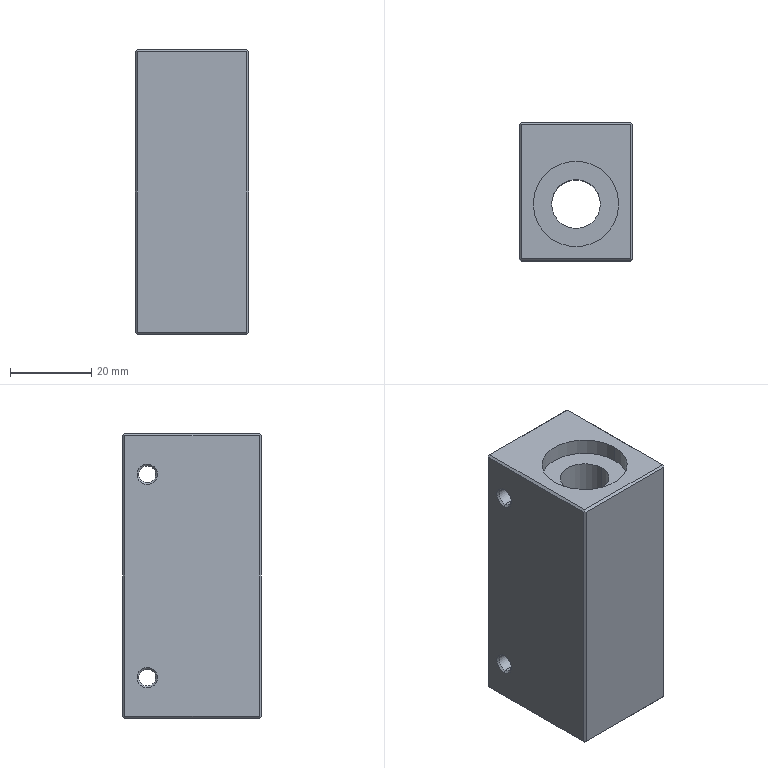Part | SolidWorks | features RevCut 7, ICE 2, Extrusion 1 | 1 solid | 50 faces | box 28 x 34 x 70 mm | volume 55264 mm3 | plane 24 | cylinder 18 | cone 8 | commonest cylinder face diameters 4.134 x4 4.917 x4 8 x4 21 x4 12 x2
STEP:
#1=CARTESIAN_POINT('',(8.,14.,22.933));
#2=VERTEX_POINT('',#1);
#3=CARTESIAN_POINT('',(8.,14.,27.067));
#4=VERTEX_POINT('',#3);
#5=CARTESIAN_POINT('',(8.,14.,25.));
#6=DIRECTION('',(-1.,0.,0.));
#7=DIRECTION('',(0.,0.,1.));
#8=AXIS2_PLACEMENT_3D('',#5,#6,#7);
#9=CIRCLE('',#8,2.067);
#10=EDGE_CURVE('',#2,#4,#9,.T.);
#11=ORIENTED_EDGE('',*,*,#10,.F.);
#12=CARTESIAN_POINT('',(-13.567,14.,22.933));
#13=VERTEX_POINT('',#12);
#14=CARTESIAN_POINT('',(8.,14.,22.933));
#15=DIRECTION('',(-1.,0.,0.));
#16=VECTOR('',#15,1000.);
#17=LINE('',#14,#16);
#18=EDGE_CURVE('',#2,#13,#17,.T.);
#19=ORIENTED_EDGE('',*,*,#18,.T.);
#20=CARTESIAN_POINT('',(-13.567,14.,27.067));
#21=VERTEX_POINT('',#20);
#22=CARTESIAN_POINT('',(-13.567,14.,25.));
#23=DIRECTION('',(-1.,0.,0.));
#24=DIRECTION('',(0.,0.,1.));
#25=AXIS2_PLACEMENT_3D('',#22,#23,#24);
#26=CIRCLE('',#25,2.067);
#27=EDGE_CURVE('',#13,#21,#26,.T.);
#28=ORIENTED_EDGE('',*,*,#27,.T.);
#29=CARTESIAN_POINT('',(8.,14.,27.067));
#30=DIRECTION('',(-1.,0.,0.));
#31=VECTOR('',#30,1000.);
#32=LINE('',#29,#31);
#33=EDGE_CURVE('',#4,#21,#32,.T.);
#34=ORIENTED_EDGE('',*,*,#33,.F.);
#35=EDGE_LOOP('',(#11,#19,#28,#34));
#36=FACE_OUTER_BOUND('',#35,.T.);
#37=CARTESIAN_POINT('',(8.,14.,25.));
#38=DIRECTION('',(-1.,0.,0.));
#39=DIRECTION('',(0.,0.,1.));
#40=AXIS2_PLACEMENT_3D('',#37,#38,#39);
#41=CYLINDRICAL_SURFACE('',#40,2.067);
#42=ADVANCED_FACE('',(#36),#41,.F.);
#43=ORIENTED_EDGE('',*,*,#27,.F.);
#44=CARTESIAN_POINT('',(-14.,14.,22.5));
#45=VERTEX_POINT('',#44);
#46=CARTESIAN_POINT('',(-13.567,14.,22.933));
#47=DIRECTION('',(-0.7071,0.,-0.7071));
#48=VECTOR('',#47,1000.);
#49=LINE('',#46,#48);
#50=EDGE_CURVE('',#13,#45,#49,.T.);
#51=ORIENTED_EDGE('',*,*,#50,.T.);
#52=CARTESIAN_POINT('',(-14.,14.,27.5));
#53=VERTEX_POINT('',#52);
#54=CARTESIAN_POINT('',(-14.,14.,25.));
#55=DIRECTION('',(-1.,0.,0.));
#56=DIRECTION('',(0.,0.,1.));
#57=AXIS2_PLACEMENT_3D('',#54,#55,#56);
#58=CIRCLE('',#57,2.5);
#59=EDGE_CURVE('',#45,#53,#58,.T.);
#60=ORIENTED_EDGE('',*,*,#59,.T.);
#61=CARTESIAN_POINT('',(-13.567,14.,27.067));
#62=DIRECTION('',(-0.7071,0.,0.7071));
#63=VECTOR('',#62,1000.);
#64=LINE('',#61,#63);
#65=EDGE_CURVE('',#21,#53,#64,.T.);
#66=ORIENTED_EDGE('',*,*,#65,.F.);
#67=EDGE_LOOP('',(#43,#51,#60,#66));
#68=FACE_OUTER_BOUND('',#67,.T.);
#69=CARTESIAN_POINT('',(-13.567,14.,25.));
#70=DIRECTION('',(-1.,0.,0.));
#71=DIRECTION('',(0.,0.,1.));
#72=AXIS2_PLACEMENT_3D('',#69,#70,#71);
#73=CONICAL_SURFACE('',#72,2.067,0.7854);
#74=ADVANCED_FACE('',(#68),#73,.F.);
#75=CARTESIAN_POINT('',(8.,14.,-27.067));
#76=VERTEX_POINT('',#75);
#77=CARTESIAN_POINT('',(8.,14.,-22.933));
#78=VERTEX_POINT('',#77);
#79=CARTESIAN_POINT('',(8.,14.,-25.));
#80=DIRECTION('',(-1.,0.,0.));
#81=DIRECTION('',(0.,0.,1.));
#82=AXIS2_PLACEMENT_3D('',#79,#80,#81);
#83=CIRCLE('',#82,2.067);
#84=EDGE_CURVE('',#76,#78,#83,.T.);
#85=ORIENTED_EDGE('',*,*,#84,.F.);
#86=CARTESIAN_POINT('',(-13.567,14.,-27.067));
#87=VERTEX_POINT('',#86);
#88=CARTESIAN_POINT('',(8.,14.,-27.067));
#89=DIRECTION('',(-1.,0.,0.));
#90=VECTOR('',#89,1000.);
#91=LINE('',#88,#90);
#92=EDGE_CURVE('',#76,#87,#91,.T.);
#93=ORIENTED_EDGE('',*,*,#92,.T.);
#94=CARTESIAN_POINT('',(-13.567,14.,-22.933));
#95=VERTEX_POINT('',#94);
#96=CARTESIAN_POINT('',(-13.567,14.,-25.));
#97=DIRECTION('',(-1.,0.,0.));
#98=DIRECTION('',(0.,0.,1.));
#99=AXIS2_PLACEMENT_3D('',#96,#97,#98);
#100=CIRCLE('',#99,2.067);
#101=EDGE_CURVE('',#87,#95,#100,.T.);
#102=ORIENTED_EDGE('',*,*,#101,.T.);
#103=CARTESIAN_POINT('',(8.,14.,-22.933));
#104=DIRECTION('',(-1.,0.,0.));
#105=VECTOR('',#104,1000.);
#106=LINE('',#103,#105);
#107=EDGE_CURVE('',#78,#95,#106,.T.);
#108=ORIENTED_EDGE('',*,*,#107,.F.);
#109=EDGE_LOOP('',(#85,#93,#102,#108));
#110=FACE_OUTER_BOUND('',#109,.T.);
#111=CARTESIAN_POINT('',(8.,14.,-25.));
#112=DIRECTION('',(-1.,0.,0.));
#113=DIRECTION('',(0.,0.,1.));
#114=AXIS2_PLACEMENT_3D('',#111,#112,#113);
#115=CYLINDRICAL_SURFACE('',#114,2.067);
#116=ADVANCED_FACE('',(#110),#115,.F.);
#117=ORIENTED_EDGE('',*,*,#101,.F.);
#118=CARTESIAN_POINT('',(-14.,14.,-27.5));
#119=VERTEX_POINT('',#118);
#120=CARTESIAN_POINT('',(-13.567,14.,-27.067));
#121=DIRECTION('',(-0.7071,0.,-0.7071));
#122=VECTOR('',#121,1000.);
#123=LINE('',#120,#122);
#124=EDGE_CURVE('',#87,#119,#123,.T.);
#125=ORIENTED_EDGE('',*,*,#124,.T.);
#126=CARTESIAN_POINT('',(-14.,14.,-22.5));
#127=VERTEX_POINT('',#126);
#128=CARTESIAN_POINT('',(-14.,14.,-25.));
#129=DIRECTION('',(-1.,0.,0.));
#130=DIRECTION('',(0.,0.,1.));
#131=AXIS2_PLACEMENT_3D('',#128,#129,#130);
#132=CIRCLE('',#131,2.5);
#133=EDGE_CURVE('',#119,#127,#132,.T.);
#134=ORIENTED_EDGE('',*,*,#133,.T.);
#135=CARTESIAN_POINT('',(-13.567,14.,-22.933));
#136=DIRECTION('',(-0.7071,0.,0.7071));
#137=VECTOR('',#136,1000.);
#138=LINE('',#135,#137);
#139=EDGE_CURVE('',#95,#127,#138,.T.);
#140=ORIENTED_EDGE('',*,*,#139,.F.);
#141=EDGE_LOOP('',(#117,#125,#134,#140));
#142=FACE_OUTER_BOUND('',#141,.T.);
#143=CARTESIAN_POINT('',(-13.567,14.,-25.));
#144=DIRECTION('',(-1.,0.,0.));
#145=DIRECTION('',(0.,0.,1.));
#146=AXIS2_PLACEMENT_3D('',#143,#144,#145);
#147=CONICAL_SURFACE('',#146,2.067,0.7854);
#148=ADVANCED_FACE('',(#142),#147,.F.);
#149=CARTESIAN_POINT('',(0.,10.92,15.541));
#150=VERTEX_POINT('',#149);
#151=CARTESIAN_POINT('',(0.,10.92,20.459));
#152=VERTEX_POINT('',#151);
#153=CARTESIAN_POINT('',(0.,10.92,18.));
#154=DIRECTION('',(0.,1.,0.));
#155=DIRECTION('',(0.,0.,1.));
#156=AXIS2_PLACEMENT_3D('',#153,#154,#155);
#157=CIRCLE('',#156,2.459);
#158=EDGE_CURVE('',#150,#152,#157,.T.);
#159=ORIENTED_EDGE('',*,*,#158,.F.);
#160=CARTESIAN_POINT('',(0.,19.459,15.541));
#161=VERTEX_POINT('',#160);
#162=CARTESIAN_POINT('',(0.,10.92,15.541));
#163=DIRECTION('',(0.,1.,0.));
#164=VECTOR('',#163,1000.);
#165=LINE('',#162,#164);
#166=EDGE_CURVE('',#150,#161,#165,.T.);
#167=ORIENTED_EDGE('',*,*,#166,.T.);
#168=CARTESIAN_POINT('',(0.,19.459,20.459));
#169=VERTEX_POINT('',#168);
#170=CARTESIAN_POINT('',(0.,19.459,18.));
#171=DIRECTION('',(0.,1.,0.));
#172=DIRECTION('',(0.,0.,1.));
#173=AXIS2_PLACEMENT_3D('',#170,#171,#172);
#174=CIRCLE('',#173,2.459);
#175=EDGE_CURVE('',#161,#169,#174,.T.);
#176=ORIENTED_EDGE('',*,*,#175,.T.);
#177=CARTESIAN_POINT('',(0.,10.92,20.459));
#178=DIRECTION('',(0.,1.,0.));
#179=VECTOR('',#178,1000.);
#180=LINE('',#177,#179);
#181=EDGE_CURVE('',#152,#169,#180,.T.);
#182=ORIENTED_EDGE('',*,*,#181,.F.);
#183=EDGE_LOOP('',(#159,#167,#176,#182));
#184=FACE_OUTER_BOUND('',#183,.T.);
#185=CARTESIAN_POINT('',(0.,10.92,18.));
#186=DIRECTION('',(0.,1.,0.));
#187=DIRECTION('',(0.,0.,1.));
#188=AXIS2_PLACEMENT_3D('',#185,#186,#187);
#189=CYLINDRICAL_SURFACE('',#188,2.459);
#190=ADVANCED_FACE('',(#184),#189,.F.);
#191=ORIENTED_EDGE('',*,*,#175,.F.);
#192=CARTESIAN_POINT('',(0.,20.,15.));
#193=VERTEX_POINT('',#192);
#194=CARTESIAN_POINT('',(0.,19.459,15.541));
#195=DIRECTION('',(0.,0.7071,-0.7071));
#196=VECTOR('',#195,1000.);
#197=LINE('',#194,#196);
#198=EDGE_CURVE('',#161,#193,#197,.T.);
#199=ORIENTED_EDGE('',*,*,#198,.T.);
#200=CARTESIAN_POINT('',(0.,20.,21.));
#201=VERTEX_POINT('',#200);
#202=CARTESIAN_POINT('',(0.,20.,18.));
#203=DIRECTION('',(0.,1.,0.));
#204=DIRECTION('',(0.,0.,1.));
#205=AXIS2_PLACEMENT_3D('',#202,#203,#204);
#206=CIRCLE('',#205,3.);
#207=EDGE_CURVE('',#193,#201,#206,.T.);
#208=ORIENTED_EDGE('',*,*,#207,.T.);
#209=CARTESIAN_POINT('',(0.,19.459,20.459));
#210=DIRECTION('',(0.,0.7071,0.7071));
#211=VECTOR('',#210,1000.);
#212=LINE('',#209,#211);
#213=EDGE_CURVE('',#169,#201,#212,.T.);
#214=ORIENTED_EDGE('',*,*,#213,.F.);
#215=EDGE_LOOP('',(#191,#199,#208,#214));
#216=FACE_OUTER_BOUND('',#215,.T.);
#217=CARTESIAN_POINT('',(0.,19.459,18.));
#218=DIRECTION('',(0.,1.,0.));
#219=DIRECTION('',(0.,0.,1.));
#220=AXIS2_PLACEMENT_3D('',#217,#218,#219);
#221=CONICAL_SURFACE('',#220,2.459,0.7854);
#222=ADVANCED_FACE('',(#216),#221,.F.);
#223=CARTESIAN_POINT('',(0.,10.92,-20.459));
#224=VERTEX_POINT('',#223);
#225=CARTESIAN_POINT('',(0.,10.92,-15.542));
#226=VERTEX_POINT('',#225);
#227=CARTESIAN_POINT('',(0.,10.92,-18.));
#228=DIRECTION('',(0.,1.,0.));
#229=DIRECTION('',(0.,0.,1.));
#230=AXIS2_PLACEMENT_3D('',#227,#228,#229);
#231=CIRCLE('',#230,2.458);
#232=EDGE_CURVE('',#224,#226,#231,.T.);
#233=ORIENTED_EDGE('',*,*,#232,.F.);
#234=CARTESIAN_POINT('',(0.,19.459,-20.459));
#235=VERTEX_POINT('',#234);
#236=CARTESIAN_POINT('',(0.,10.92,-20.459));
#237=DIRECTION('',(0.,1.,0.));
#238=VECTOR('',#237,1000.);
#239=LINE('',#236,#238);
#240=EDGE_CURVE('',#224,#235,#239,.T.);
#241=ORIENTED_EDGE('',*,*,#240,.T.);
#242=CARTESIAN_POINT('',(0.,19.459,-15.542));
#243=VERTEX_POINT('',#242);
#244=CARTESIAN_POINT('',(0.,19.459,-18.));
#245=DIRECTION('',(0.,1.,0.));
#246=DIRECTION('',(0.,0.,1.));
#247=AXIS2_PLACEMENT_3D('',#244,#245,#246);
#248=CIRCLE('',#247,2.458);
#249=EDGE_CURVE('',#235,#243,#248,.T.);
#250=ORIENTED_EDGE('',*,*,#249,.T.);
#251=CARTESIAN_POINT('',(0.,10.92,-15.542));
#252=DIRECTION('',(0.,1.,0.));
#253=VECTOR('',#252,1000.);
#254=LINE('',#251,#253);
#255=EDGE_CURVE('',#226,#243,#254,.T.);
#256=ORIENTED_EDGE('',*,*,#255,.F.);
#257=EDGE_LOOP('',(#233,#241,#250,#256));
#258=FACE_OUTER_BOUND('',#257,.T.);
#259=CARTESIAN_POINT('',(0.,10.92,-18.));
#260=DIRECTION('',(0.,1.,0.));
#261=DIRECTION('',(0.,0.,1.));
#262=AXIS2_PLACEMENT_3D('',#259,#260,#261);
#263=CYLINDRICAL_SURFACE('',#262,2.458);
#264=ADVANCED_FACE('',(#258),#263,.F.);
#265=ORIENTED_EDGE('',*,*,#249,.F.);
#266=CARTESIAN_POINT('',(0.,20.,-21.));
#267=VERTEX_POINT('',#266);
#268=CARTESIAN_POINT('',(0.,19.459,-20.459));
#269=DIRECTION('',(0.,0.7071,-0.7071));
#270=VECTOR('',#269,1000.);
#271=LINE('',#268,#270);
#272=EDGE_CURVE('',#235,#267,#271,.T.);
#273=ORIENTED_EDGE('',*,*,#272,.T.);
#274=CARTESIAN_POINT('',(0.,20.,-15.));
#275=VERTEX_POINT('',#274);
#276=CARTESIAN_POINT('',(0.,20.,-18.));
#277=DIRECTION('',(0.,1.,0.));
#278=DIRECTION('',(0.,0.,1.));
#279=AXIS2_PLACEMENT_3D('',#276,#277,#278);
#280=CIRCLE('',#279,3.);
#281=EDGE_CURVE('',#267,#275,#280,.T.);
#282=ORIENTED_EDGE('',*,*,#281,.T.);
#283=CARTESIAN_POINT('',(0.,19.459,-15.542));
#284=DIRECTION('',(0.,0.7071,0.7071));
#285=VECTOR('',#284,1000.);
#286=LINE('',#283,#285);
#287=EDGE_CURVE('',#243,#275,#286,.T.);
#288=ORIENTED_EDGE('',*,*,#287,.F.);
#289=EDGE_LOOP('',(#265,#273,#282,#288));
#290=FACE_OUTER_BOUND('',#289,.T.);
#291=CARTESIAN_POINT('',(0.,19.459,-18.));
#292=DIRECTION('',(0.,1.,0.));
#293=DIRECTION('',(0.,0.,1.));
#294=AXIS2_PLACEMENT_3D('',#291,#292,#293);
#295=CONICAL_SURFACE('',#294,2.458,0.7854);
#296=ADVANCED_FACE('',(#290),#295,.F.);
#297=CARTESIAN_POINT('',(14.,14.,-29.));
#298=VERTEX_POINT('',#297);
#299=CARTESIAN_POINT('',(14.,14.,-21.));
#300=VERTEX_POINT('',#299);
#301=CARTESIAN_POINT('',(14.,14.,-25.));
#302=DIRECTION('',(-1.,0.,0.));
#303=DIRECTION('',(0.,0.,1.));
#304=AXIS2_PLACEMENT_3D('',#301,#302,#303);
#305=CIRCLE('',#304,4.);
#306=EDGE_CURVE('',#298,#300,#305,.T.);
#307=ORIENTED_EDGE('',*,*,#306,.F.);
#308=CARTESIAN_POINT('',(8.,14.,-29.));
#309=VERTEX_POINT('',#308);
#310=CARTESIAN_POINT('',(14.,14.,-29.));
#311=DIRECTION('',(-1.,0.,0.));
#312=VECTOR('',#311,1000.);
#313=LINE('',#310,#312);
#314=EDGE_CURVE('',#298,#309,#313,.T.);
#315=ORIENTED_EDGE('',*,*,#314,.T.);
#316=CARTESIAN_POINT('',(8.,14.,-21.));
#317=VERTEX_POINT('',#316);
#318=CARTESIAN_POINT('',(8.,14.,-25.));
#319=DIRECTION('',(-1.,0.,0.));
#320=DIRECTION('',(0.,0.,1.));
#321=AXIS2_PLACEMENT_3D('',#318,#319,#320);
#322=CIRCLE('',#321,4.);
#323=EDGE_CURVE('',#309,#317,#322,.T.);
#324=ORIENTED_EDGE('',*,*,#323,.T.);
#325=CARTESIAN_POINT('',(14.,14.,-21.));
#326=DIRECTION('',(-1.,0.,0.));
#327=VECTOR('',#326,1000.);
#328=LINE('',#325,#327);
#329=EDGE_CURVE('',#300,#317,#328,.T.);
#330=ORIENTED_EDGE('',*,*,#329,.F.);
#331=EDGE_LOOP('',(#307,#315,#324,#330));
#332=FACE_OUTER_BOUND('',#331,.T.);
#333=CARTESIAN_POINT('',(14.,14.,-25.));
#334=DIRECTION('',(-1.,0.,0.));
#335=DIRECTION('',(0.,0.,1.));
#336=AXIS2_PLACEMENT_3D('',#333,#334,#335);
#337=CYLINDRICAL_SURFACE('',#336,4.);
#338=ADVANCED_FACE('',(#332),#337,.F.);
#339=CARTESIAN_POINT('',(14.,14.,21.));
#340=VERTEX_POINT('',#339);
#341=CARTESIAN_POINT('',(14.,14.,29.));
#342=VERTEX_POINT('',#341);
#343=CARTESIAN_POINT('',(14.,14.,25.));
#344=DIRECTION('',(-1.,0.,0.));
#345=DIRECTION('',(0.,0.,1.));
#346=AXIS2_PLACEMENT_3D('',#343,#344,#345);
#347=CIRCLE('',#346,4.);
#348=EDGE_CURVE('',#340,#342,#347,.T.);
#349=ORIENTED_EDGE('',*,*,#348,.F.);
#350=CARTESIAN_POINT('',(8.,14.,21.));
#351=VERTEX_POINT('',#350);
#352=CARTESIAN_POINT('',(14.,14.,21.));
#353=DIRECTION('',(-1.,0.,0.));
#354=VECTOR('',#353,1000.);
#355=LINE('',#352,#354);
#356=EDGE_CURVE('',#340,#351,#355,.T.);
#357=ORIENTED_EDGE('',*,*,#356,.T.);
#358=CARTESIAN_POINT('',(8.,14.,29.));
#359=VERTEX_POINT('',#358);
#360=CARTESIAN_POINT('',(8.,14.,25.));
#361=DIRECTION('',(-1.,0.,0.));
#362=DIRECTION('',(0.,0.,1.));
#363=AXIS2_PLACEMENT_3D('',#360,#361,#362);
#364=CIRCLE('',#363,4.);
#365=EDGE_CURVE('',#351,#359,#364,.T.);
#366=ORIENTED_EDGE('',*,*,#365,.T.);
#367=CARTESIAN_POINT('',(14.,14.,29.));
#368=DIRECTION('',(-1.,0.,0.));
#369=VECTOR('',#368,1000.);
#370=LINE('',#367,#369);
#371=EDGE_CURVE('',#342,#359,#370,.T.);
#372=ORIENTED_EDGE('',*,*,#371,.F.);
#373=EDGE_LOOP('',(#349,#357,#366,#372));
#374=FACE_OUTER_BOUND('',#373,.T.);
#375=CARTESIAN_POINT('',(14.,14.,25.));
#376=DIRECTION('',(-1.,0.,0.));
#377=DIRECTION('',(0.,0.,1.));
#378=AXIS2_PLACEMENT_3D('',#375,#376,#377);
#379=CYLINDRICAL_SURFACE('',#378,4.);
#380=ADVANCED_FACE('',(#374),#379,.F.);
#381=CARTESIAN_POINT('',(-10.5,0.,-35.));
#382=VERTEX_POINT('',#381);
#383=CARTESIAN_POINT('',(10.5,0.,-35.));
#384=VERTEX_POINT('',#383);
#385=CARTESIAN_POINT('',(0.,0.,-35.));
#386=DIRECTION('',(0.,0.,1.));
#387=DIRECTION('',(1.,0.,0.));
#388=AXIS2_PLACEMENT_3D('',#385,#386,#387);
#389=CIRCLE('',#388,10.5);
#390=EDGE_CURVE('',#382,#384,#389,.T.);
#391=ORIENTED_EDGE('',*,*,#390,.F.);
#392=CARTESIAN_POINT('',(-10.5,0.,-31.04));
#393=VERTEX_POINT('',#392);
#394=CARTESIAN_POINT('',(-10.5,0.,-35.));
#395=DIRECTION('',(0.,0.,1.));
#396=VECTOR('',#395,1000.);
#397=LINE('',#394,#396);
#398=EDGE_CURVE('',#382,#393,#397,.T.);
#399=ORIENTED_EDGE('',*,*,#398,.T.);
#400=CARTESIAN_POINT('',(10.5,0.,-31.04));
#401=VERTEX_POINT('',#400);
#402=CARTESIAN_POINT('',(0.,0.,-31.04));
#403=DIRECTION('',(0.,0.,1.));
#404=DIRECTION('',(1.,0.,0.));
#405=AXIS2_PLACEMENT_3D('',#402,#403,#404);
#406=CIRCLE('',#405,10.5);
#407=EDGE_CURVE('',#393,#401,#406,.T.);
#408=ORIENTED_EDGE('',*,*,#407,.T.);
#409=CARTESIAN_POINT('',(10.5,0.,-35.));
#410=DIRECTION('',(0.,0.,1.));
#411=VECTOR('',#410,1000.);
#412=LINE('',#409,#411);
#413=EDGE_CURVE('',#384,#401,#412,.T.);
#414=ORIENTED_EDGE('',*,*,#413,.F.);
#415=EDGE_LOOP('',(#391,#399,#408,#414));
#416=FACE_OUTER_BOUND('',#415,.T.);
#417=CARTESIAN_POINT('',(0.,0.,-35.));
#418=DIRECTION('',(0.,0.,1.));
#419=DIRECTION('',(1.,0.,0.));
#420=AXIS2_PLACEMENT_3D('',#417,#418,#419);
#421=CYLINDRICAL_SURFACE('',#420,10.5);
#422=ADVANCED_FACE('',(#416),#421,.F.);
#423=CARTESIAN_POINT('',(-6.,0.,-31.04));
#424=VERTEX_POINT('',#423);
#425=CARTESIAN_POINT('',(6.,0.,-31.04));
#426=VERTEX_POINT('',#425);
#427=CARTESIAN_POINT('',(0.,0.,-31.04));
#428=DIRECTION('',(0.,0.,1.));
#429=DIRECTION('',(1.,0.,0.));
#430=AXIS2_PLACEMENT_3D('',#427,#428,#429);
#431=CIRCLE('',#430,6.);
#432=EDGE_CURVE('',#424,#426,#431,.T.);
#433=ORIENTED_EDGE('',*,*,#432,.F.);
#434=CARTESIAN_POINT('',(-6.,0.,31.04));
#435=VERTEX_POINT('',#434);
#436=CARTESIAN_POINT('',(-6.,0.,-35.));
#437=DIRECTION('',(0.,0.,1.));
#438=VECTOR('',#437,1000.);
#439=LINE('',#436,#438);
#440=EDGE_CURVE('',#424,#435,#439,.T.);
#441=ORIENTED_EDGE('',*,*,#440,.T.);
#442=CARTESIAN_POINT('',(6.,0.,31.04));
#443=VERTEX_POINT('',#442);
#444=CARTESIAN_POINT('',(0.,0.,31.04));
#445=DIRECTION('',(0.,0.,1.));
#446=DIRECTION('',(1.,0.,0.));
#447=AXIS2_PLACEMENT_3D('',#444,#445,#446);
#448=CIRCLE('',#447,6.);
#449=EDGE_CURVE('',#435,#443,#448,.T.);
#450=ORIENTED_EDGE('',*,*,#449,.T.);
#451=CARTESIAN_POINT('',(6.,0.,-35.));
#452=DIRECTION('',(0.,0.,1.));
#453=VECTOR('',#452,1000.);
#454=LINE('',#451,#453);
#455=EDGE_CURVE('',#426,#443,#454,.T.);
#456=ORIENTED_EDGE('',*,*,#455,.F.);
#457=EDGE_LOOP('',(#433,#441,#450,#456));
#458=FACE_OUTER_BOUND('',#457,.T.);
#459=CARTESIAN_POINT('',(0.,0.,-35.));
#460=DIRECTION('',(0.,0.,1.));
#461=DIRECTION('',(1.,0.,0.));
#462=AXIS2_PLACEMENT_3D('',#459,#460,#461);
#463=CYLINDRICAL_SURFACE('',#462,6.);
#464=ADVANCED_FACE('',(#458),#463,.F.);
#465=CARTESIAN_POINT('',(-10.5,0.,31.04));
#466=VERTEX_POINT('',#465);
#467=CARTESIAN_POINT('',(10.5,0.,31.04));
#468=VERTEX_POINT('',#467);
#469=CARTESIAN_POINT('',(0.,0.,31.04));
#470=DIRECTION('',(0.,0.,1.));
#471=DIRECTION('',(1.,0.,0.));
#472=AXIS2_PLACEMENT_3D('',#469,#470,#471);
#473=CIRCLE('',#472,10.5);
#474=EDGE_CURVE('',#466,#468,#473,.T.);
#475=ORIENTED_EDGE('',*,*,#474,.F.);
#476=CARTESIAN_POINT('',(-10.5,0.,35.));
#477=VERTEX_POINT('',#476);
#478=CARTESIAN_POINT('',(-10.5,0.,-35.));
#479=DIRECTION('',(0.,0.,1.));
#480=VECTOR('',#479,1000.);
#481=LINE('',#478,#480);
#482=EDGE_CURVE('',#466,#477,#481,.T.);
#483=ORIENTED_EDGE('',*,*,#482,.T.);
#484=CARTESIAN_POINT('',(10.5,0.,35.));
#485=VERTEX_POINT('',#484);
#486=CARTESIAN_POINT('',(0.,0.,35.));
#487=DIRECTION('',(0.,0.,1.));
#488=DIRECTION('',(1.,0.,0.));
#489=AXIS2_PLACEMENT_3D('',#486,#487,#488);
#490=CIRCLE('',#489,10.5);
#491=EDGE_CURVE('',#477,#485,#490,.T.);
#492=ORIENTED_EDGE('',*,*,#491,.T.);
#493=CARTESIAN_POINT('',(10.5,0.,-35.));
#494=DIRECTION('',(0.,0.,1.));
#495=VECTOR('',#494,1000.);
#496=LINE('',#493,#495);
#497=EDGE_CURVE('',#468,#485,#496,.T.);
#498=ORIENTED_EDGE('',*,*,#497,.F.);
#499=EDGE_LOOP('',(#475,#483,#492,#498));
#500=FACE_OUTER_BOUND('',#499,.T.);
#501=CARTESIAN_POINT('',(0.,0.,-35.));
#502=DIRECTION('',(0.,0.,1.));
#503=DIRECTION('',(1.,0.,0.));
#504=AXIS2_PLACEMENT_3D('',#501,#502,#503);
#505=CYLINDRICAL_SURFACE('',#504,10.5);
#506=ADVANCED_FACE('',(#500),#505,.F.);
#507=CARTESIAN_POINT('',(-14.,14.,-25.));
#508=DIRECTION('',(-1.,0.,0.));
#509=DIRECTION('',(0.,0.,1.));
#510=AXIS2_PLACEMENT_3D('',#507,#508,#509);
#511=CIRCLE('',#510,2.5);
#512=EDGE_CURVE('',#127,#119,#511,.T.);
#513=ORIENTED_EDGE('',*,*,#512,.F.);
#514=ORIENTED_EDGE('',*,*,#133,.F.);
#515=EDGE_LOOP('',(#513,#514));
#516=FACE_BOUND('',#515,.T.);
#517=CARTESIAN_POINT('',(-14.,14.,25.));
#518=DIRECTION('',(-1.,0.,0.));
#519=DIRECTION('',(0.,0.,1.));
#520=AXIS2_PLACEMENT_3D('',#517,#518,#519);
#521=CIRCLE('',#520,2.5);
#522=EDGE_CURVE('',#53,#45,#521,.T.);
#523=ORIENTED_EDGE('',*,*,#522,.F.);
#524=ORIENTED_EDGE('',*,*,#59,.F.);
#525=EDGE_LOOP('',(#523,#524));
#526=FACE_BOUND('',#525,.T.);
#527=CARTESIAN_POINT('',(-14.,-13.5,-34.5));
#528=VERTEX_POINT('',#527);
#529=CARTESIAN_POINT('',(-14.,19.5,-34.5));
#530=VERTEX_POINT('',#529);
#531=CARTESIAN_POINT('',(-14.,-34.,-34.5));
#532=DIRECTION('',(0.,1.,0.));
#533=VECTOR('',#532,1000.);
#534=LINE('',#531,#533);
#535=EDGE_CURVE('',#528,#530,#534,.T.);
#536=ORIENTED_EDGE('',*,*,#535,.F.);
#537=CARTESIAN_POINT('',(-14.,-13.5,34.5));
#538=VERTEX_POINT('',#537);
#539=CARTESIAN_POINT('',(-14.,-13.5,-35.));
#540=DIRECTION('',(0.,0.,1.));
#541=VECTOR('',#540,1000.);
#542=LINE('',#539,#541);
#543=EDGE_CURVE('',#528,#538,#542,.T.);
#544=ORIENTED_EDGE('',*,*,#543,.T.);
#545=CARTESIAN_POINT('',(-14.,19.5,34.5));
#546=VERTEX_POINT('',#545);
#547=CARTESIAN_POINT('',(-14.,-34.,34.5));
#548=DIRECTION('',(0.,1.,0.));
#549=VECTOR('',#548,1000.);
#550=LINE('',#547,#549);
#551=EDGE_CURVE('',#538,#546,#550,.T.);
#552=ORIENTED_EDGE('',*,*,#551,.T.);
#553=CARTESIAN_POINT('',(-14.,19.5,-35.));
#554=DIRECTION('',(0.,0.,1.));
#555=VECTOR('',#554,1000.);
#556=LINE('',#553,#555);
#557=EDGE_CURVE('',#530,#546,#556,.T.);
#558=ORIENTED_EDGE('',*,*,#557,.F.);
#559=EDGE_LOOP('',(#536,#544,#552,#558));
#560=FACE_OUTER_BOUND('',#559,.T.);
#561=CARTESIAN_POINT('',(-14.,0.,0.));
#562=DIRECTION('',(1.,0.,0.));
#563=DIRECTION('',(0.,0.,-1.));
#564=AXIS2_PLACEMENT_3D('',#561,#562,#563);
#565=PLANE('',#564);
#566=ADVANCED_FACE('',(#516,#526,#560),#565,.F.);
#567=CARTESIAN_POINT('',(14.,14.,25.));
#568=DIRECTION('',(-1.,0.,0.));
#569=DIRECTION('',(0.,0.,1.));
#570=AXIS2_PLACEMENT_3D('',#567,#568,#569);
#571=CIRCLE('',#570,4.);
#572=EDGE_CURVE('',#342,#340,#571,.T.);
#573=ORIENTED_EDGE('',*,*,#572,.T.);
#574=ORIENTED_EDGE('',*,*,#348,.T.);
#575=EDGE_LOOP('',(#573,#574));
#576=FACE_BOUND('',#575,.T.);
#577=CARTESIAN_POINT('',(14.,14.,-25.));
#578=DIRECTION('',(-1.,0.,0.));
#579=DIRECTION('',(0.,0.,1.));
#580=AXIS2_PLACEMENT_3D('',#577,#578,#579);
#581=CIRCLE('',#580,4.);
#582=EDGE_CURVE('',#300,#298,#581,.T.);
#583=ORIENTED_EDGE('',*,*,#582,.T.);
#584=ORIENTED_EDGE('',*,*,#306,.T.);
#585=EDGE_LOOP('',(#583,#584));
#586=FACE_BOUND('',#585,.T.);
#587=CARTESIAN_POINT('',(14.,-13.5,-34.5));
#588=VERTEX_POINT('',#587);
#589=CARTESIAN_POINT('',(14.,-13.5,34.5));
#590=VERTEX_POINT('',#589);
#591=CARTESIAN_POINT('',(14.,-13.5,-35.));
#592=DIRECTION('',(0.,0.,1.));
#593=VECTOR('',#592,1000.);
#594=LINE('',#591,#593);
#595=EDGE_CURVE('',#588,#590,#594,.T.);
#596=ORIENTED_EDGE('',*,*,#595,.F.);
#597=CARTESIAN_POINT('',(14.,19.5,-34.5));
#598=VERTEX_POINT('',#597);
#599=CARTESIAN_POINT('',(14.,-34.,-34.5));
#600=DIRECTION('',(0.,1.,0.));
#601=VECTOR('',#600,1000.);
#602=LINE('',#599,#601);
#603=EDGE_CURVE('',#588,#598,#602,.T.);
#604=ORIENTED_EDGE('',*,*,#603,.T.);
#605=CARTESIAN_POINT('',(14.,19.5,34.5));
#606=VERTEX_POINT('',#605);
#607=CARTESIAN_POINT('',(14.,19.5,-35.));
#608=DIRECTION('',(0.,0.,1.));
#609=VECTOR('',#608,1000.);
#610=LINE('',#607,#609);
#611=EDGE_CURVE('',#598,#606,#610,.T.);
#612=ORIENTED_EDGE('',*,*,#611,.T.);
#613=CARTESIAN_POINT('',(14.,-34.,34.5));
#614=DIRECTION('',(0.,1.,0.));
#615=VECTOR('',#614,1000.);
#616=LINE('',#613,#615);
#617=EDGE_CURVE('',#590,#606,#616,.T.);
#618=ORIENTED_EDGE('',*,*,#617,.F.);
#619=EDGE_LOOP('',(#596,#604,#612,#618));
#620=FACE_OUTER_BOUND('',#619,.T.);
#621=CARTESIAN_POINT('',(14.,0.,0.));
#622=DIRECTION('',(1.,0.,0.));
#623=DIRECTION('',(0.,0.,-1.));
#624=AXIS2_PLACEMENT_3D('',#621,#622,#623);
#625=PLANE('',#624);
#626=ADVANCED_FACE('',(#576,#586,#620),#625,.T.);
#627=CARTESIAN_POINT('',(13.5,-13.5,35.));
#628=VERTEX_POINT('',#627);
#629=CARTESIAN_POINT('',(13.75,-13.75,34.75));
#630=VERTEX_POINT('',#629);
#631=CARTESIAN_POINT('',(13.667,-13.667,34.833));
#632=DIRECTION('',(0.5774,-0.5774,-0.5774));
#633=VECTOR('',#632,1000.);
#634=LINE('',#631,#633);
#635=EDGE_CURVE('',#628,#630,#634,.T.);
#636=ORIENTED_EDGE('',*,*,#635,.F.);
#637=CARTESIAN_POINT('',(-13.5,-13.5,35.));
#638=VERTEX_POINT('',#637);
#639=CARTESIAN_POINT('',(14.,-13.5,35.));
#640=DIRECTION('',(-1.,0.,0.));
#641=VECTOR('',#640,1000.);
#642=LINE('',#639,#641);
#643=EDGE_CURVE('',#628,#638,#642,.T.);
#644=ORIENTED_EDGE('',*,*,#643,.T.);
#645=CARTESIAN_POINT('',(-13.75,-13.75,34.75));
#646=VERTEX_POINT('',#645);
#647=CARTESIAN_POINT('',(-4.333,-4.333,44.167));
#648=DIRECTION('',(0.5774,0.5774,0.5774));
#649=VECTOR('',#648,1000.);
#650=LINE('',#647,#649);
#651=EDGE_CURVE('',#646,#638,#650,.T.);
#652=ORIENTED_EDGE('',*,*,#651,.F.);
#653=CARTESIAN_POINT('',(-13.5,-14.,34.5));
#654=VERTEX_POINT('',#653);
#655=CARTESIAN_POINT('',(-4.667,-22.833,25.667));
#656=DIRECTION('',(-0.5774,0.5774,0.5774));
#657=VECTOR('',#656,1000.);
#658=LINE('',#655,#657);
#659=EDGE_CURVE('',#654,#646,#658,.T.);
#660=ORIENTED_EDGE('',*,*,#659,.F.);
#661=CARTESIAN_POINT('',(13.5,-14.,34.5));
#662=VERTEX_POINT('',#661);
#663=CARTESIAN_POINT('',(14.,-14.,34.5));
#664=DIRECTION('',(-1.,0.,0.));
#665=VECTOR('',#664,1000.);
#666=LINE('',#663,#665);
#667=EDGE_CURVE('',#662,#654,#666,.T.);
#668=ORIENTED_EDGE('',*,*,#667,.F.);
#669=CARTESIAN_POINT('',(14.,-13.5,35.));
#670=DIRECTION('',(-0.5774,-0.5774,-0.5774));
#671=VECTOR('',#670,1000.);
#672=LINE('',#669,#671);
#673=EDGE_CURVE('',#630,#662,#672,.T.);
#674=ORIENTED_EDGE('',*,*,#673,.F.);
#675=EDGE_LOOP('',(#636,#644,#652,#660,#668,#674));
#676=FACE_OUTER_BOUND('',#675,.T.);
#677=CARTESIAN_POINT('',(14.,-13.5,35.));
#678=DIRECTION('',(0.,0.7071,-0.7071));
#679=DIRECTION('',(0.,0.7071,0.7071));
#680=AXIS2_PLACEMENT_3D('',#677,#678,#679);
#681=PLANE('',#680);
#682=ADVANCED_FACE('',(#676),#681,.F.);
#683=CARTESIAN_POINT('',(-13.5,-13.5,-35.));
#684=VERTEX_POINT('',#683);
#685=CARTESIAN_POINT('',(-13.75,-13.75,-34.75));
#686=VERTEX_POINT('',#685);
#687=CARTESIAN_POINT('',(-4.667,-4.667,-43.833));
#688=DIRECTION('',(-0.5774,-0.5774,0.5774));
#689=VECTOR('',#688,1000.);
#690=LINE('',#687,#689);
#691=EDGE_CURVE('',#684,#686,#690,.T.);
#692=ORIENTED_EDGE('',*,*,#691,.F.);
#693=CARTESIAN_POINT('',(13.5,-13.5,-35.));
#694=VERTEX_POINT('',#693);
#695=CARTESIAN_POINT('',(14.,-13.5,-35.));
#696=DIRECTION('',(-1.,0.,0.));
#697=VECTOR('',#696,1000.);
#698=LINE('',#695,#697);
#699=EDGE_CURVE('',#694,#684,#698,.T.);
#700=ORIENTED_EDGE('',*,*,#699,.F.);
#701=CARTESIAN_POINT('',(13.75,-13.75,-34.75));
#702=VERTEX_POINT('',#701);
#703=CARTESIAN_POINT('',(14.,-14.,-34.5));
#704=DIRECTION('',(-0.5774,0.5774,-0.5774));
#705=VECTOR('',#704,1000.);
#706=LINE('',#703,#705);
#707=EDGE_CURVE('',#702,#694,#706,.T.);
#708=ORIENTED_EDGE('',*,*,#707,.F.);
#709=CARTESIAN_POINT('',(13.5,-14.,-34.5));
#710=VERTEX_POINT('',#709);
#711=CARTESIAN_POINT('',(13.667,-13.833,-34.667));
#712=DIRECTION('',(0.5774,0.5774,-0.5774));
#713=VECTOR('',#712,1000.);
#714=LINE('',#711,#713);
#715=EDGE_CURVE('',#710,#702,#714,.T.);
#716=ORIENTED_EDGE('',*,*,#715,.F.);
#717=CARTESIAN_POINT('',(-13.5,-14.,-34.5));
#718=VERTEX_POINT('',#717);
#719=CARTESIAN_POINT('',(14.,-14.,-34.5));
#720=DIRECTION('',(-1.,0.,0.));
#721=VECTOR('',#720,1000.);
#722=LINE('',#719,#721);
#723=EDGE_CURVE('',#710,#718,#722,.T.);
#724=ORIENTED_EDGE('',*,*,#723,.T.);
#725=CARTESIAN_POINT('',(-4.333,-23.167,-25.333));
#726=DIRECTION('',(0.5774,-0.5774,0.5774));
#727=VECTOR('',#726,1000.);
#728=LINE('',#725,#727);
#729=EDGE_CURVE('',#686,#718,#728,.T.);
#730=ORIENTED_EDGE('',*,*,#729,.F.);
#731=EDGE_LOOP('',(#692,#700,#708,#716,#724,#730));
#732=FACE_OUTER_BOUND('',#731,.T.);
#733=CARTESIAN_POINT('',(14.,-14.,-34.5));
#734=DIRECTION('',(0.,0.7071,0.7071));
#735=DIRECTION('',(0.,-0.7071,0.7071));
#736=AXIS2_PLACEMENT_3D('',#733,#734,#735);
#737=PLANE('',#736);
#738=ADVANCED_FACE('',(#732),#737,.F.);
#739=CARTESIAN_POINT('',(-13.75,19.75,-34.75));
#740=VERTEX_POINT('',#739);
#741=CARTESIAN_POINT('',(-13.5,19.5,-35.));
#742=VERTEX_POINT('',#741);
#743=CARTESIAN_POINT('',(-4.333,10.333,-44.167));
#744=DIRECTION('',(0.5774,-0.5774,-0.5774));
#745=VECTOR('',#744,1000.);
#746=LINE('',#743,#745);
#747=EDGE_CURVE('',#740,#742,#746,.T.);
#748=ORIENTED_EDGE('',*,*,#747,.F.);
#749=CARTESIAN_POINT('',(-13.5,20.,-34.5));
#750=VERTEX_POINT('',#749);
#751=CARTESIAN_POINT('',(-4.667,28.833,-25.667));
#752=DIRECTION('',(-0.5774,-0.5774,-0.5774));
#753=VECTOR('',#752,1000.);
#754=LINE('',#751,#753);
#755=EDGE_CURVE('',#750,#740,#754,.T.);
#756=ORIENTED_EDGE('',*,*,#755,.F.);
#757=CARTESIAN_POINT('',(13.5,20.,-34.5));
#758=VERTEX_POINT('',#757);
#759=CARTESIAN_POINT('',(14.,20.,-34.5));
#760=DIRECTION('',(-1.,0.,0.));
#761=VECTOR('',#760,1000.);
#762=LINE('',#759,#761);
#763=EDGE_CURVE('',#758,#750,#762,.T.);
#764=ORIENTED_EDGE('',*,*,#763,.F.);
#765=CARTESIAN_POINT('',(13.75,19.75,-34.75));
#766=VERTEX_POINT('',#765);
#767=CARTESIAN_POINT('',(14.,19.5,-35.));
#768=DIRECTION('',(-0.5774,0.5774,0.5774));
#769=VECTOR('',#768,1000.);
#770=LINE('',#767,#769);
#771=EDGE_CURVE('',#766,#758,#770,.T.);
#772=ORIENTED_EDGE('',*,*,#771,.F.);
#773=CARTESIAN_POINT('',(13.5,19.5,-35.));
#774=VERTEX_POINT('',#773);
#775=CARTESIAN_POINT('',(13.667,19.667,-34.833));
#776=DIRECTION('',(0.5774,0.5774,0.5774));
#777=VECTOR('',#776,1000.);
#778=LINE('',#775,#777);
#779=EDGE_CURVE('',#774,#766,#778,.T.);
#780=ORIENTED_EDGE('',*,*,#779,.F.);
#781=CARTESIAN_POINT('',(14.,19.5,-35.));
#782=DIRECTION('',(-1.,0.,0.));
#783=VECTOR('',#782,1000.);
#784=LINE('',#781,#783);
#785=EDGE_CURVE('',#774,#742,#784,.T.);
#786=ORIENTED_EDGE('',*,*,#785,.T.);
#787=EDGE_LOOP('',(#748,#756,#764,#772,#780,#786));
#788=FACE_OUTER_BOUND('',#787,.T.);
#789=CARTESIAN_POINT('',(14.,19.5,-35.));
#790=DIRECTION('',(0.,-0.7071,0.7071));
#791=DIRECTION('',(0.,-0.7071,-0.7071));
#792=AXIS2_PLACEMENT_3D('',#789,#790,#791);
#793=PLANE('',#792);
#794=ADVANCED_FACE('',(#788),#793,.F.);
#795=CARTESIAN_POINT('',(13.75,19.75,34.75));
#796=VERTEX_POINT('',#795);
#797=CARTESIAN_POINT('',(13.5,19.5,35.));
#798=VERTEX_POINT('',#797);
#799=CARTESIAN_POINT('',(14.,20.,34.5));
#800=DIRECTION('',(-0.5774,-0.5774,0.5774));
#801=VECTOR('',#800,1000.);
#802=LINE('',#799,#801);
#803=EDGE_CURVE('',#796,#798,#802,.T.);
#804=ORIENTED_EDGE('',*,*,#803,.F.);
#805=CARTESIAN_POINT('',(13.5,20.,34.5));
#806=VERTEX_POINT('',#805);
#807=CARTESIAN_POINT('',(13.667,19.833,34.667));
#808=DIRECTION('',(0.5774,-0.5774,0.5774));
#809=VECTOR('',#808,1000.);
#810=LINE('',#807,#809);
#811=EDGE_CURVE('',#806,#796,#810,.T.);
#812=ORIENTED_EDGE('',*,*,#811,.F.);
#813=CARTESIAN_POINT('',(-13.5,20.,34.5));
#814=VERTEX_POINT('',#813);
#815=CARTESIAN_POINT('',(14.,20.,34.5));
#816=DIRECTION('',(-1.,0.,0.));
#817=VECTOR('',#816,1000.);
#818=LINE('',#815,#817);
#819=EDGE_CURVE('',#806,#814,#818,.T.);
#820=ORIENTED_EDGE('',*,*,#819,.T.);
#821=CARTESIAN_POINT('',(-13.75,19.75,34.75));
#822=VERTEX_POINT('',#821);
#823=CARTESIAN_POINT('',(-4.333,29.167,25.333));
#824=DIRECTION('',(0.5774,0.5774,-0.5774));
#825=VECTOR('',#824,1000.);
#826=LINE('',#823,#825);
#827=EDGE_CURVE('',#822,#814,#826,.T.);
#828=ORIENTED_EDGE('',*,*,#827,.F.);
#829=CARTESIAN_POINT('',(-13.5,19.5,35.));
#830=VERTEX_POINT('',#829);
#831=CARTESIAN_POINT('',(-4.667,10.667,43.833));
#832=DIRECTION('',(-0.5774,0.5774,-0.5774));
#833=VECTOR('',#832,1000.);
#834=LINE('',#831,#833);
#835=EDGE_CURVE('',#830,#822,#834,.T.);
#836=ORIENTED_EDGE('',*,*,#835,.F.);
#837=CARTESIAN_POINT('',(14.,19.5,35.));
#838=DIRECTION('',(-1.,0.,0.));
#839=VECTOR('',#838,1000.);
#840=LINE('',#837,#839);
#841=EDGE_CURVE('',#798,#830,#840,.T.);
#842=ORIENTED_EDGE('',*,*,#841,.F.);
#843=EDGE_LOOP('',(#804,#812,#820,#828,#836,#842));
#844=FACE_OUTER_BOUND('',#843,.T.);
#845=CARTESIAN_POINT('',(14.,20.,34.5));
#846=DIRECTION('',(0.,-0.7071,-0.7071));
#847=DIRECTION('',(0.,0.7071,-0.7071));
#848=AXIS2_PLACEMENT_3D('',#845,#846,#847);
#849=PLANE('',#848);
#850=ADVANCED_FACE('',(#844),#849,.F.);
#851=CARTESIAN_POINT('',(0.,0.,35.));
#852=DIRECTION('',(0.,0.,1.));
#853=DIRECTION('',(1.,0.,0.));
#854=AXIS2_PLACEMENT_3D('',#851,#852,#853);
#855=CIRCLE('',#854,10.5);
#856=EDGE_CURVE('',#485,#477,#855,.T.);
#857=ORIENTED_EDGE('',*,*,#856,.F.);
#858=ORIENTED_EDGE('',*,*,#491,.F.);
#859=EDGE_LOOP('',(#857,#858));
#860=FACE_BOUND('',#859,.T.);
#861=CARTESIAN_POINT('',(13.5,-34.,35.));
#862=DIRECTION('',(0.,1.,0.));
#863=VECTOR('',#862,1000.);
#864=LINE('',#861,#863);
#865=EDGE_CURVE('',#628,#798,#864,.T.);
#866=ORIENTED_EDGE('',*,*,#865,.T.);
#867=ORIENTED_EDGE('',*,*,#841,.T.);
#868=CARTESIAN_POINT('',(-13.5,-34.,35.));
#869=DIRECTION('',(0.,1.,0.));
#870=VECTOR('',#869,1000.);
#871=LINE('',#868,#870);
#872=EDGE_CURVE('',#638,#830,#871,.T.);
#873=ORIENTED_EDGE('',*,*,#872,.F.);
#874=ORIENTED_EDGE('',*,*,#643,.F.);
#875=EDGE_LOOP('',(#866,#867,#873,#874));
#876=FACE_OUTER_BOUND('',#875,.T.);
#877=CARTESIAN_POINT('',(14.,19.5,35.));
#878=DIRECTION('',(0.,0.,-1.));
#879=DIRECTION('',(-1.,0.,0.));
#880=AXIS2_PLACEMENT_3D('',#877,#878,#879);
#881=PLANE('',#880);
#882=ADVANCED_FACE('',(#860,#876),#881,.F.);
#883=CARTESIAN_POINT('',(0.,0.,-35.));
#884=DIRECTION('',(0.,0.,1.));
#885=DIRECTION('',(1.,0.,0.));
#886=AXIS2_PLACEMENT_3D('',#883,#884,#885);
#887=CIRCLE('',#886,10.5);
#888=EDGE_CURVE('',#384,#382,#887,.T.);
#889=ORIENTED_EDGE('',*,*,#888,.T.);
#890=ORIENTED_EDGE('',*,*,#390,.T.);
#891=EDGE_LOOP('',(#889,#890));
#892=FACE_BOUND('',#891,.T.);
#893=CARTESIAN_POINT('',(-13.5,-34.,-35.));
#894=DIRECTION('',(0.,1.,0.));
#895=VECTOR('',#894,1000.);
#896=LINE('',#893,#895);
#897=EDGE_CURVE('',#684,#742,#896,.T.);
#898=ORIENTED_EDGE('',*,*,#897,.T.);
#899=ORIENTED_EDGE('',*,*,#785,.F.);
#900=CARTESIAN_POINT('',(13.5,-34.,-35.));
#901=DIRECTION('',(0.,1.,0.));
#902=VECTOR('',#901,1000.);
#903=LINE('',#900,#902);
#904=EDGE_CURVE('',#694,#774,#903,.T.);
#905=ORIENTED_EDGE('',*,*,#904,.F.);
#906=ORIENTED_EDGE('',*,*,#699,.T.);
#907=EDGE_LOOP('',(#898,#899,#905,#906));
#908=FACE_OUTER_BOUND('',#907,.T.);
#909=CARTESIAN_POINT('',(14.,-13.5,-35.));
#910=DIRECTION('',(0.,0.,1.));
#911=DIRECTION('',(1.,0.,0.));
#912=AXIS2_PLACEMENT_3D('',#909,#910,#911);
#913=PLANE('',#912);
#914=ADVANCED_FACE('',(#892,#908),#913,.F.);
#915=ORIENTED_EDGE('',*,*,#611,.F.);
#916=CARTESIAN_POINT('',(13.833,19.667,-34.667));
#917=DIRECTION('',(-0.5774,0.5774,-0.5774));
#918=VECTOR('',#917,1000.);
#919=LINE('',#916,#918);
#920=EDGE_CURVE('',#598,#766,#919,.T.);
#921=ORIENTED_EDGE('',*,*,#920,.T.);
#922=ORIENTED_EDGE('',*,*,#771,.T.);
#923=CARTESIAN_POINT('',(13.5,20.,-35.));
#924=DIRECTION('',(0.,0.,1.));
#925=VECTOR('',#924,1000.);
#926=LINE('',#923,#925);
#927=EDGE_CURVE('',#758,#806,#926,.T.);
#928=ORIENTED_EDGE('',*,*,#927,.T.);
#929=ORIENTED_EDGE('',*,*,#811,.T.);
#930=CARTESIAN_POINT('',(37.167,-3.667,11.333));
#931=DIRECTION('',(0.5774,-0.5774,-0.5774));
#932=VECTOR('',#931,1000.);
#933=LINE('',#930,#932);
#934=EDGE_CURVE('',#796,#606,#933,.T.);
#935=ORIENTED_EDGE('',*,*,#934,.T.);
#936=EDGE_LOOP('',(#915,#921,#922,#928,#929,#935));
#937=FACE_OUTER_BOUND('',#936,.T.);
#938=CARTESIAN_POINT('',(14.,19.5,-35.));
#939=DIRECTION('',(0.7071,0.7071,0.));
#940=DIRECTION('',(-0.7071,0.7071,0.));
#941=AXIS2_PLACEMENT_3D('',#938,#939,#940);
#942=PLANE('',#941);
#943=ADVANCED_FACE('',(#937),#942,.T.);
#944=ORIENTED_EDGE('',*,*,#755,.T.);
#945=CARTESIAN_POINT('',(-13.5,20.,-35.));
#946=DIRECTION('',(-0.5774,-0.5774,0.5774));
#947=VECTOR('',#946,1000.);
#948=LINE('',#945,#947);
#949=EDGE_CURVE('',#740,#530,#948,.T.);
#950=ORIENTED_EDGE('',*,*,#949,.T.);
#951=ORIENTED_EDGE('',*,*,#557,.T.);
#952=CARTESIAN_POINT('',(-36.833,-3.333,11.667));
#953=DIRECTION('',(0.5774,0.5774,0.5774));
#954=VECTOR('',#953,1000.);
#955=LINE('',#952,#954);
#956=EDGE_CURVE('',#546,#822,#955,.T.);
#957=ORIENTED_EDGE('',*,*,#956,.T.);
#958=ORIENTED_EDGE('',*,*,#827,.T.);
#959=CARTESIAN_POINT('',(-13.5,20.,-35.));
#960=DIRECTION('',(0.,0.,1.));
#961=VECTOR('',#960,1000.);
#962=LINE('',#959,#961);
#963=EDGE_CURVE('',#750,#814,#962,.T.);
#964=ORIENTED_EDGE('',*,*,#963,.F.);
#965=EDGE_LOOP('',(#944,#950,#951,#957,#958,#964));
#966=FACE_OUTER_BOUND('',#965,.T.);
#967=CARTESIAN_POINT('',(-13.5,20.,-35.));
#968=DIRECTION('',(-0.7071,0.7071,0.));
#969=DIRECTION('',(-0.7071,-0.7071,0.));
#970=AXIS2_PLACEMENT_3D('',#967,#968,#969);
#971=PLANE('',#970);
#972=ADVANCED_FACE('',(#966),#971,.T.);
#973=ORIENTED_EDGE('',*,*,#543,.F.);
#974=CARTESIAN_POINT('',(-13.833,-13.667,-34.667));
#975=DIRECTION('',(0.5774,-0.5774,-0.5774));
#976=VECTOR('',#975,1000.);
#977=LINE('',#974,#976);
#978=EDGE_CURVE('',#528,#686,#977,.T.);
#979=ORIENTED_EDGE('',*,*,#978,.T.);
#980=ORIENTED_EDGE('',*,*,#729,.T.);
#981=CARTESIAN_POINT('',(-13.5,-14.,-35.));
#982=DIRECTION('',(0.,0.,1.));
#983=VECTOR('',#982,1000.);
#984=LINE('',#981,#983);
#985=EDGE_CURVE('',#718,#654,#984,.T.);
#986=ORIENTED_EDGE('',*,*,#985,.T.);
#987=ORIENTED_EDGE('',*,*,#659,.T.);
#988=CARTESIAN_POINT('',(-37.167,9.667,11.333));
#989=DIRECTION('',(-0.5774,0.5774,-0.5774));
#990=VECTOR('',#989,1000.);
#991=LINE('',#988,#990);
#992=EDGE_CURVE('',#646,#538,#991,.T.);
#993=ORIENTED_EDGE('',*,*,#992,.T.);
#994=EDGE_LOOP('',(#973,#979,#980,#986,#987,#993));
#995=FACE_OUTER_BOUND('',#994,.T.);
#996=CARTESIAN_POINT('',(-14.,-13.5,-35.));
#997=DIRECTION('',(-0.7071,-0.7071,0.));
#998=DIRECTION('',(0.7071,-0.7071,0.));
#999=AXIS2_PLACEMENT_3D('',#996,#997,#998);
#1000=PLANE('',#999);
#1001=ADVANCED_FACE('',(#995),#1000,.T.);
#1002=ORIENTED_EDGE('',*,*,#715,.T.);
#1003=CARTESIAN_POINT('',(13.5,-14.,-35.));
#1004=DIRECTION('',(0.5774,0.5774,0.5774));
#1005=VECTOR('',#1004,1000.);
#1006=LINE('',#1003,#1005);
#1007=EDGE_CURVE('',#702,#588,#1006,.T.);
#1008=ORIENTED_EDGE('',*,*,#1007,.T.);
#1009=ORIENTED_EDGE('',*,*,#595,.T.);
#1010=CARTESIAN_POINT('',(36.833,9.333,11.667));
#1011=DIRECTION('',(-0.5774,-0.5774,0.5774));
#1012=VECTOR('',#1011,1000.);
#1013=LINE('',#1010,#1012);
#1014=EDGE_CURVE('',#590,#630,#1013,.T.);
#1015=ORIENTED_EDGE('',*,*,#1014,.T.);
#1016=ORIENTED_EDGE('',*,*,#673,.T.);
#1017=CARTESIAN_POINT('',(13.5,-14.,-35.));
#1018=DIRECTION('',(0.,0.,1.));
#1019=VECTOR('',#1018,1000.);
#1020=LINE('',#1017,#1019);
#1021=EDGE_CURVE('',#710,#662,#1020,.T.);
#1022=ORIENTED_EDGE('',*,*,#1021,.F.);
#1023=EDGE_LOOP('',(#1002,#1008,#1009,#1015,#1016,#1022));
#1024=FACE_OUTER_BOUND('',#1023,.T.);
#1025=CARTESIAN_POINT('',(13.5,-14.,-35.));
#1026=DIRECTION('',(0.7071,-0.7071,0.));
#1027=DIRECTION('',(0.7071,0.7071,0.));
#1028=AXIS2_PLACEMENT_3D('',#1025,#1026,#1027);
#1029=PLANE('',#1028);
#1030=ADVANCED_FACE('',(#1024),#1029,.T.);
#1031=CARTESIAN_POINT('',(0.,20.,-18.));
#1032=DIRECTION('',(0.,1.,0.));
#1033=DIRECTION('',(0.,0.,1.));
#1034=AXIS2_PLACEMENT_3D('',#1031,#1032,#1033);
#1035=CIRCLE('',#1034,3.);
#1036=EDGE_CURVE('',#275,#267,#1035,.T.);
#1037=ORIENTED_EDGE('',*,*,#1036,.F.);
#1038=ORIENTED_EDGE('',*,*,#281,.F.);
#1039=EDGE_LOOP('',(#1037,#1038));
#1040=FACE_BOUND('',#1039,.T.);
#1041=CARTESIAN_POINT('',(0.,20.,18.));
#1042=DIRECTION('',(0.,1.,0.));
#1043=DIRECTION('',(0.,0.,1.));
#1044=AXIS2_PLACEMENT_3D('',#1041,#1042,#1043);
#1045=CIRCLE('',#1044,3.);
#1046=EDGE_CURVE('',#201,#193,#1045,.T.);
#1047=ORIENTED_EDGE('',*,*,#1046,.F.);
#1048=ORIENTED_EDGE('',*,*,#207,.F.);
#1049=EDGE_LOOP('',(#1047,#1048));
#1050=FACE_BOUND('',#1049,.T.);
#1051=ORIENTED_EDGE('',*,*,#963,.T.);
#1052=ORIENTED_EDGE('',*,*,#819,.F.);
#1053=ORIENTED_EDGE('',*,*,#927,.F.);
#1054=ORIENTED_EDGE('',*,*,#763,.T.);
#1055=EDGE_LOOP('',(#1051,#1052,#1053,#1054));
#1056=FACE_OUTER_BOUND('',#1055,.T.);
#1057=CARTESIAN_POINT('',(14.,20.,-34.5));
#1058=DIRECTION('',(0.,-1.,0.));
#1059=DIRECTION('',(0.,0.,-1.));
#1060=AXIS2_PLACEMENT_3D('',#1057,#1058,#1059);
#1061=PLANE('',#1060);
#1062=ADVANCED_FACE('',(#1040,#1050,#1056),#1061,.F.);
#1063=ORIENTED_EDGE('',*,*,#1021,.T.);
#1064=ORIENTED_EDGE('',*,*,#667,.T.);
#1065=ORIENTED_EDGE('',*,*,#985,.F.);
#1066=ORIENTED_EDGE('',*,*,#723,.F.);
#1067=EDGE_LOOP('',(#1063,#1064,#1065,#1066));
#1068=FACE_OUTER_BOUND('',#1067,.T.);
#1069=CARTESIAN_POINT('',(14.,-14.,34.5));
#1070=DIRECTION('',(0.,1.,0.));
#1071=DIRECTION('',(0.,0.,1.));
#1072=AXIS2_PLACEMENT_3D('',#1069,#1070,#1071);
#1073=PLANE('',#1072);
#1074=ADVANCED_FACE('',(#1068),#1073,.F.);
#1075=CARTESIAN_POINT('',(8.,14.,25.));
#1076=DIRECTION('',(-1.,0.,0.));
#1077=DIRECTION('',(0.,0.,1.));
#1078=AXIS2_PLACEMENT_3D('',#1075,#1076,#1077);
#1079=CIRCLE('',#1078,4.);
#1080=EDGE_CURVE('',#359,#351,#1079,.T.);
#1081=ORIENTED_EDGE('',*,*,#1080,.F.);
#1082=ORIENTED_EDGE('',*,*,#365,.F.);
#1083=EDGE_LOOP('',(#1081,#1082));
#1084=FACE_OUTER_BOUND('',#1083,.T.);
#1085=CARTESIAN_POINT('',(8.,14.,25.));
#1086=DIRECTION('',(-1.,0.,0.));
#1087=DIRECTION('',(0.,0.,1.));
#1088=AXIS2_PLACEMENT_3D('',#1085,#1086,#1087);
#1089=CIRCLE('',#1088,2.067);
#1090=EDGE_CURVE('',#4,#2,#1089,.T.);
#1091=ORIENTED_EDGE('',*,*,#1090,.T.);
#1092=ORIENTED_EDGE('',*,*,#10,.T.);
#1093=EDGE_LOOP('',(#1091,#1092));
#1094=FACE_BOUND('',#1093,.T.);
#1095=CARTESIAN_POINT('',(8.,14.,25.));
#1096=DIRECTION('',(1.,0.,0.));
#1097=DIRECTION('',(0.,0.,-1.));
#1098=AXIS2_PLACEMENT_3D('',#1095,#1096,#1097);
#1099=PLANE('',#1098);
#1100=ADVANCED_FACE('',(#1084,#1094),#1099,.T.);
#1101=CARTESIAN_POINT('',(8.,14.,-25.));
#1102=DIRECTION('',(-1.,0.,0.));
#1103=DIRECTION('',(0.,0.,1.));
#1104=AXIS2_PLACEMENT_3D('',#1101,#1102,#1103);
#1105=CIRCLE('',#1104,4.);
#1106=EDGE_CURVE('',#317,#309,#1105,.T.);
#1107=ORIENTED_EDGE('',*,*,#1106,.F.);
#1108=ORIENTED_EDGE('',*,*,#323,.F.);
#1109=EDGE_LOOP('',(#1107,#1108));
#1110=FACE_OUTER_BOUND('',#1109,.T.);
#1111=CARTESIAN_POINT('',(8.,14.,-25.));
#1112=DIRECTION('',(-1.,0.,0.));
#1113=DIRECTION('',(0.,0.,1.));
#1114=AXIS2_PLACEMENT_3D('',#1111,#1112,#1113);
#1115=CIRCLE('',#1114,2.067);
#1116=EDGE_CURVE('',#78,#76,#1115,.T.);
#1117=ORIENTED_EDGE('',*,*,#1116,.T.);
#1118=ORIENTED_EDGE('',*,*,#84,.T.);
#1119=EDGE_LOOP('',(#1117,#1118));
#1120=FACE_BOUND('',#1119,.T.);
#1121=CARTESIAN_POINT('',(8.,14.,-25.));
#1122=DIRECTION('',(1.,0.,0.));
#1123=DIRECTION('',(0.,0.,-1.));
#1124=AXIS2_PLACEMENT_3D('',#1121,#1122,#1123);
#1125=PLANE('',#1124);
#1126=ADVANCED_FACE('',(#1110,#1120),#1125,.T.);
#1127=ORIENTED_EDGE('',*,*,#482,.F.);
#1128=CARTESIAN_POINT('',(0.,0.,31.04));
#1129=DIRECTION('',(0.,0.,1.));
#1130=DIRECTION('',(1.,0.,0.));
#1131=AXIS2_PLACEMENT_3D('',#1128,#1129,#1130);
#1132=CIRCLE('',#1131,10.5);
#1133=EDGE_CURVE('',#468,#466,#1132,.T.);
#1134=ORIENTED_EDGE('',*,*,#1133,.F.);
#1135=ORIENTED_EDGE('',*,*,#497,.T.);
#1136=ORIENTED_EDGE('',*,*,#856,.T.);
#1137=EDGE_LOOP('',(#1127,#1134,#1135,#1136));
#1138=FACE_OUTER_BOUND('',#1137,.T.);
#1139=CARTESIAN_POINT('',(0.,0.,-35.));
#1140=DIRECTION('',(0.,0.,1.));
#1141=DIRECTION('',(1.,0.,0.));
#1142=AXIS2_PLACEMENT_3D('',#1139,#1140,#1141);
#1143=CYLINDRICAL_SURFACE('',#1142,10.5);
#1144=ADVANCED_FACE('',(#1138),#1143,.F.);
#1145=ORIENTED_EDGE('',*,*,#1133,.T.);
#1146=ORIENTED_EDGE('',*,*,#474,.T.);
#1147=EDGE_LOOP('',(#1145,#1146));
#1148=FACE_OUTER_BOUND('',#1147,.T.);
#1149=CARTESIAN_POINT('',(0.,0.,31.04));
#1150=DIRECTION('',(0.,0.,1.));
#1151=DIRECTION('',(1.,0.,0.));
#1152=AXIS2_PLACEMENT_3D('',#1149,#1150,#1151);
#1153=CIRCLE('',#1152,6.);
#1154=EDGE_CURVE('',#443,#435,#1153,.T.);
#1155=ORIENTED_EDGE('',*,*,#1154,.F.);
#1156=ORIENTED_EDGE('',*,*,#449,.F.);
#1157=EDGE_LOOP('',(#1155,#1156));
#1158=FACE_BOUND('',#1157,.T.);
#1159=CARTESIAN_POINT('',(0.,10.5,31.04));
#1160=DIRECTION('',(0.,0.,1.));
#1161=DIRECTION('',(1.,0.,0.));
#1162=AXIS2_PLACEMENT_3D('',#1159,#1160,#1161);
#1163=PLANE('',#1162);
#1164=ADVANCED_FACE('',(#1148,#1158),#1163,.T.);
#1165=ORIENTED_EDGE('',*,*,#440,.F.);
#1166=CARTESIAN_POINT('',(0.,0.,-31.04));
#1167=DIRECTION('',(0.,0.,1.));
#1168=DIRECTION('',(1.,0.,0.));
#1169=AXIS2_PLACEMENT_3D('',#1166,#1167,#1168);
#1170=CIRCLE('',#1169,6.);
#1171=EDGE_CURVE('',#426,#424,#1170,.T.);
#1172=ORIENTED_EDGE('',*,*,#1171,.F.);
#1173=ORIENTED_EDGE('',*,*,#455,.T.);
#1174=ORIENTED_EDGE('',*,*,#1154,.T.);
#1175=EDGE_LOOP('',(#1165,#1172,#1173,#1174));
#1176=FACE_OUTER_BOUND('',#1175,.T.);
#1177=CARTESIAN_POINT('',(0.,0.,-35.));
#1178=DIRECTION('',(0.,0.,1.));
#1179=DIRECTION('',(1.,0.,0.));
#1180=AXIS2_PLACEMENT_3D('',#1177,#1178,#1179);
#1181=CYLINDRICAL_SURFACE('',#1180,6.);
#1182=ADVANCED_FACE('',(#1176),#1181,.F.);
#1183=ORIENTED_EDGE('',*,*,#1171,.T.);
#1184=ORIENTED_EDGE('',*,*,#432,.T.);
#1185=EDGE_LOOP('',(#1183,#1184));
#1186=FACE_BOUND('',#1185,.T.);
#1187=CARTESIAN_POINT('',(0.,0.,-31.04));
#1188=DIRECTION('',(0.,0.,1.));
#1189=DIRECTION('',(1.,0.,0.));
#1190=AXIS2_PLACEMENT_3D('',#1187,#1188,#1189);
#1191=CIRCLE('',#1190,10.5);
#1192=EDGE_CURVE('',#401,#393,#1191,.T.);
#1193=ORIENTED_EDGE('',*,*,#1192,.F.);
#1194=ORIENTED_EDGE('',*,*,#407,.F.);
#1195=EDGE_LOOP('',(#1193,#1194));
#1196=FACE_OUTER_BOUND('',#1195,.T.);
#1197=CARTESIAN_POINT('',(0.,6.,-31.04));
#1198=DIRECTION('',(0.,0.,-1.));
#1199=DIRECTION('',(-1.,0.,0.));
#1200=AXIS2_PLACEMENT_3D('',#1197,#1198,#1199);
#1201=PLANE('',#1200);
#1202=ADVANCED_FACE('',(#1186,#1196),#1201,.T.);
#1203=ORIENTED_EDGE('',*,*,#398,.F.);
#1204=ORIENTED_EDGE('',*,*,#888,.F.);
#1205=ORIENTED_EDGE('',*,*,#413,.T.);
#1206=ORIENTED_EDGE('',*,*,#1192,.T.);
#1207=EDGE_LOOP('',(#1203,#1204,#1205,#1206));
#1208=FACE_OUTER_BOUND('',#1207,.T.);
#1209=CARTESIAN_POINT('',(0.,0.,-35.));
#1210=DIRECTION('',(0.,0.,1.));
#1211=DIRECTION('',(1.,0.,0.));
#1212=AXIS2_PLACEMENT_3D('',#1209,#1210,#1211);
#1213=CYLINDRICAL_SURFACE('',#1212,10.5);
#1214=ADVANCED_FACE('',(#1208),#1213,.F.);
#1215=ORIENTED_EDGE('',*,*,#356,.F.);
#1216=ORIENTED_EDGE('',*,*,#572,.F.);
#1217=ORIENTED_EDGE('',*,*,#371,.T.);
#1218=ORIENTED_EDGE('',*,*,#1080,.T.);
#1219=EDGE_LOOP('',(#1215,#1216,#1217,#1218));
#1220=FACE_OUTER_BOUND('',#1219,.T.);
#1221=CARTESIAN_POINT('',(14.,14.,25.));
#1222=DIRECTION('',(-1.,0.,0.));
#1223=DIRECTION('',(0.,0.,1.));
#1224=AXIS2_PLACEMENT_3D('',#1221,#1222,#1223);
#1225=CYLINDRICAL_SURFACE('',#1224,4.);
#1226=ADVANCED_FACE('',(#1220),#1225,.F.);
#1227=ORIENTED_EDGE('',*,*,#314,.F.);
#1228=ORIENTED_EDGE('',*,*,#582,.F.);
#1229=ORIENTED_EDGE('',*,*,#329,.T.);
#1230=ORIENTED_EDGE('',*,*,#1106,.T.);
#1231=EDGE_LOOP('',(#1227,#1228,#1229,#1230));
#1232=FACE_OUTER_BOUND('',#1231,.T.);
#1233=CARTESIAN_POINT('',(14.,14.,-25.));
#1234=DIRECTION('',(-1.,0.,0.));
#1235=DIRECTION('',(0.,0.,1.));
#1236=AXIS2_PLACEMENT_3D('',#1233,#1234,#1235);
#1237=CYLINDRICAL_SURFACE('',#1236,4.);
#1238=ADVANCED_FACE('',(#1232),#1237,.F.);
#1239=ORIENTED_EDGE('',*,*,#272,.F.);
#1240=CARTESIAN_POINT('',(0.,19.459,-18.));
#1241=DIRECTION('',(0.,1.,0.));
#1242=DIRECTION('',(0.,0.,1.));
#1243=AXIS2_PLACEMENT_3D('',#1240,#1241,#1242);
#1244=CIRCLE('',#1243,2.458);
#1245=EDGE_CURVE('',#243,#235,#1244,.T.);
#1246=ORIENTED_EDGE('',*,*,#1245,.F.);
#1247=ORIENTED_EDGE('',*,*,#287,.T.);
#1248=ORIENTED_EDGE('',*,*,#1036,.T.);
#1249=EDGE_LOOP('',(#1239,#1246,#1247,#1248));
#1250=FACE_OUTER_BOUND('',#1249,.T.);
#1251=CARTESIAN_POINT('',(0.,19.459,-18.));
#1252=DIRECTION('',(0.,1.,0.));
#1253=DIRECTION('',(0.,0.,1.));
#1254=AXIS2_PLACEMENT_3D('',#1251,#1252,#1253);
#1255=CONICAL_SURFACE('',#1254,2.458,0.7854);
#1256=ADVANCED_FACE('',(#1250),#1255,.F.);
#1257=ORIENTED_EDGE('',*,*,#240,.F.);
#1258=CARTESIAN_POINT('',(0.,10.92,-18.));
#1259=DIRECTION('',(0.,1.,0.));
#1260=DIRECTION('',(0.,0.,1.));
#1261=AXIS2_PLACEMENT_3D('',#1258,#1259,#1260);
#1262=CIRCLE('',#1261,2.458);
#1263=EDGE_CURVE('',#226,#224,#1262,.T.);
#1264=ORIENTED_EDGE('',*,*,#1263,.F.);
#1265=ORIENTED_EDGE('',*,*,#255,.T.);
#1266=ORIENTED_EDGE('',*,*,#1245,.T.);
#1267=EDGE_LOOP('',(#1257,#1264,#1265,#1266));
#1268=FACE_OUTER_BOUND('',#1267,.T.);
#1269=CARTESIAN_POINT('',(0.,10.92,-18.));
#1270=DIRECTION('',(0.,1.,0.));
#1271=DIRECTION('',(0.,0.,1.));
#1272=AXIS2_PLACEMENT_3D('',#1269,#1270,#1271);
#1273=CYLINDRICAL_SURFACE('',#1272,2.458);
#1274=ADVANCED_FACE('',(#1268),#1273,.F.);
#1275=ORIENTED_EDGE('',*,*,#1263,.T.);
#1276=ORIENTED_EDGE('',*,*,#232,.T.);
#1277=EDGE_LOOP('',(#1275,#1276));
#1278=FACE_OUTER_BOUND('',#1277,.T.);
#1279=CARTESIAN_POINT('',(0.,10.92,-20.459));
#1280=DIRECTION('',(0.,1.,0.));
#1281=DIRECTION('',(0.,0.,1.));
#1282=AXIS2_PLACEMENT_3D('',#1279,#1280,#1281);
#1283=PLANE('',#1282);
#1284=ADVANCED_FACE('',(#1278),#1283,.T.);
#1285=ORIENTED_EDGE('',*,*,#198,.F.);
#1286=CARTESIAN_POINT('',(0.,19.459,18.));
#1287=DIRECTION('',(0.,1.,0.));
#1288=DIRECTION('',(0.,0.,1.));
#1289=AXIS2_PLACEMENT_3D('',#1286,#1287,#1288);
#1290=CIRCLE('',#1289,2.459);
#1291=EDGE_CURVE('',#169,#161,#1290,.T.);
#1292=ORIENTED_EDGE('',*,*,#1291,.F.);
#1293=ORIENTED_EDGE('',*,*,#213,.T.);
#1294=ORIENTED_EDGE('',*,*,#1046,.T.);
#1295=EDGE_LOOP('',(#1285,#1292,#1293,#1294));
#1296=FACE_OUTER_BOUND('',#1295,.T.);
#1297=CARTESIAN_POINT('',(0.,19.459,18.));
#1298=DIRECTION('',(0.,1.,0.));
#1299=DIRECTION('',(0.,0.,1.));
#1300=AXIS2_PLACEMENT_3D('',#1297,#1298,#1299);
#1301=CONICAL_SURFACE('',#1300,2.459,0.7854);
#1302=ADVANCED_FACE('',(#1296),#1301,.F.);
#1303=ORIENTED_EDGE('',*,*,#166,.F.);
#1304=CARTESIAN_POINT('',(0.,10.92,18.));
#1305=DIRECTION('',(0.,1.,0.));
#1306=DIRECTION('',(0.,0.,1.));
#1307=AXIS2_PLACEMENT_3D('',#1304,#1305,#1306);
#1308=CIRCLE('',#1307,2.459);
#1309=EDGE_CURVE('',#152,#150,#1308,.T.);
#1310=ORIENTED_EDGE('',*,*,#1309,.F.);
#1311=ORIENTED_EDGE('',*,*,#181,.T.);
#1312=ORIENTED_EDGE('',*,*,#1291,.T.);
#1313=EDGE_LOOP('',(#1303,#1310,#1311,#1312));
#1314=FACE_OUTER_BOUND('',#1313,.T.);
#1315=CARTESIAN_POINT('',(0.,10.92,18.));
#1316=DIRECTION('',(0.,1.,0.));
#1317=DIRECTION('',(0.,0.,1.));
#1318=AXIS2_PLACEMENT_3D('',#1315,#1316,#1317);
#1319=CYLINDRICAL_SURFACE('',#1318,2.459);
#1320=ADVANCED_FACE('',(#1314),#1319,.F.);
#1321=ORIENTED_EDGE('',*,*,#1309,.T.);
#1322=ORIENTED_EDGE('',*,*,#158,.T.);
#1323=EDGE_LOOP('',(#1321,#1322));
#1324=FACE_OUTER_BOUND('',#1323,.T.);
#1325=CARTESIAN_POINT('',(0.,10.92,15.541));
#1326=DIRECTION('',(0.,1.,0.));
#1327=DIRECTION('',(0.,0.,1.));
#1328=AXIS2_PLACEMENT_3D('',#1325,#1326,#1327);
#1329=PLANE('',#1328);
#1330=ADVANCED_FACE('',(#1324),#1329,.T.);
#1331=ORIENTED_EDGE('',*,*,#124,.F.);
#1332=CARTESIAN_POINT('',(-13.567,14.,-25.));
#1333=DIRECTION('',(-1.,0.,0.));
#1334=DIRECTION('',(0.,0.,1.));
#1335=AXIS2_PLACEMENT_3D('',#1332,#1333,#1334);
#1336=CIRCLE('',#1335,2.067);
#1337=EDGE_CURVE('',#95,#87,#1336,.T.);
#1338=ORIENTED_EDGE('',*,*,#1337,.F.);
#1339=ORIENTED_EDGE('',*,*,#139,.T.);
#1340=ORIENTED_EDGE('',*,*,#512,.T.);
#1341=EDGE_LOOP('',(#1331,#1338,#1339,#1340));
#1342=FACE_OUTER_BOUND('',#1341,.T.);
#1343=CARTESIAN_POINT('',(-13.567,14.,-25.));
#1344=DIRECTION('',(-1.,0.,0.));
#1345=DIRECTION('',(0.,0.,1.));
#1346=AXIS2_PLACEMENT_3D('',#1343,#1344,#1345);
#1347=CONICAL_SURFACE('',#1346,2.067,0.7854);
#1348=ADVANCED_FACE('',(#1342),#1347,.F.);
#1349=ORIENTED_EDGE('',*,*,#92,.F.);
#1350=ORIENTED_EDGE('',*,*,#1116,.F.);
#1351=ORIENTED_EDGE('',*,*,#107,.T.);
#1352=ORIENTED_EDGE('',*,*,#1337,.T.);
#1353=EDGE_LOOP('',(#1349,#1350,#1351,#1352));
#1354=FACE_OUTER_BOUND('',#1353,.T.);
#1355=CARTESIAN_POINT('',(8.,14.,-25.));
#1356=DIRECTION('',(-1.,0.,0.));
#1357=DIRECTION('',(0.,0.,1.));
#1358=AXIS2_PLACEMENT_3D('',#1355,#1356,#1357);
#1359=CYLINDRICAL_SURFACE('',#1358,2.067);
#1360=ADVANCED_FACE('',(#1354),#1359,.F.);
#1361=ORIENTED_EDGE('',*,*,#50,.F.);
#1362=CARTESIAN_POINT('',(-13.567,14.,25.));
#1363=DIRECTION('',(-1.,0.,0.));
#1364=DIRECTION('',(0.,0.,1.));
#1365=AXIS2_PLACEMENT_3D('',#1362,#1363,#1364);
#1366=CIRCLE('',#1365,2.067);
#1367=EDGE_CURVE('',#21,#13,#1366,.T.);
#1368=ORIENTED_EDGE('',*,*,#1367,.F.);
#1369=ORIENTED_EDGE('',*,*,#65,.T.);
#1370=ORIENTED_EDGE('',*,*,#522,.T.);
#1371=EDGE_LOOP('',(#1361,#1368,#1369,#1370));
#1372=FACE_OUTER_BOUND('',#1371,.T.);
#1373=CARTESIAN_POINT('',(-13.567,14.,25.));
#1374=DIRECTION('',(-1.,0.,0.));
#1375=DIRECTION('',(0.,0.,1.));
#1376=AXIS2_PLACEMENT_3D('',#1373,#1374,#1375);
#1377=CONICAL_SURFACE('',#1376,2.067,0.7854);
#1378=ADVANCED_FACE('',(#1372),#1377,.F.);
#1379=ORIENTED_EDGE('',*,*,#18,.F.);
#1380=ORIENTED_EDGE('',*,*,#1090,.F.);
#1381=ORIENTED_EDGE('',*,*,#33,.T.);
#1382=ORIENTED_EDGE('',*,*,#1367,.T.);
#1383=EDGE_LOOP('',(#1379,#1380,#1381,#1382));
#1384=FACE_OUTER_BOUND('',#1383,.T.);
#1385=CARTESIAN_POINT('',(8.,14.,25.));
#1386=DIRECTION('',(-1.,0.,0.));
#1387=DIRECTION('',(0.,0.,1.));
#1388=AXIS2_PLACEMENT_3D('',#1385,#1386,#1387);
#1389=CYLINDRICAL_SURFACE('',#1388,2.067);
#1390=ADVANCED_FACE('',(#1384),#1389,.F.);
#1391=ORIENTED_EDGE('',*,*,#803,.T.);
#1392=ORIENTED_EDGE('',*,*,#865,.F.);
#1393=ORIENTED_EDGE('',*,*,#635,.T.);
#1394=ORIENTED_EDGE('',*,*,#1014,.F.);
#1395=ORIENTED_EDGE('',*,*,#617,.T.);
#1396=ORIENTED_EDGE('',*,*,#934,.F.);
#1397=EDGE_LOOP('',(#1391,#1392,#1393,#1394,#1395,#1396));
#1398=FACE_OUTER_BOUND('',#1397,.T.);
#1399=CARTESIAN_POINT('',(13.5,-34.,35.));
#1400=DIRECTION('',(0.7071,0.,0.7071));
#1401=DIRECTION('',(0.7071,0.,-0.7071));
#1402=AXIS2_PLACEMENT_3D('',#1399,#1400,#1401);
#1403=PLANE('',#1402);
#1404=ADVANCED_FACE('',(#1398),#1403,.T.);
#1405=ORIENTED_EDGE('',*,*,#779,.T.);
#1406=ORIENTED_EDGE('',*,*,#920,.F.);
#1407=ORIENTED_EDGE('',*,*,#603,.F.);
#1408=ORIENTED_EDGE('',*,*,#1007,.F.);
#1409=ORIENTED_EDGE('',*,*,#707,.T.);
#1410=ORIENTED_EDGE('',*,*,#904,.T.);
#1411=EDGE_LOOP('',(#1405,#1406,#1407,#1408,#1409,#1410));
#1412=FACE_OUTER_BOUND('',#1411,.T.);
#1413=CARTESIAN_POINT('',(14.,-34.,-34.5));
#1414=DIRECTION('',(0.7071,0.,-0.7071));
#1415=DIRECTION('',(-0.7071,0.,-0.7071));
#1416=AXIS2_PLACEMENT_3D('',#1413,#1414,#1415);
#1417=PLANE('',#1416);
#1418=ADVANCED_FACE('',(#1412),#1417,.T.);
#1419=ORIENTED_EDGE('',*,*,#835,.T.);
#1420=ORIENTED_EDGE('',*,*,#956,.F.);
#1421=ORIENTED_EDGE('',*,*,#551,.F.);
#1422=ORIENTED_EDGE('',*,*,#992,.F.);
#1423=ORIENTED_EDGE('',*,*,#651,.T.);
#1424=ORIENTED_EDGE('',*,*,#872,.T.);
#1425=EDGE_LOOP('',(#1419,#1420,#1421,#1422,#1423,#1424));
#1426=FACE_OUTER_BOUND('',#1425,.T.);
#1427=CARTESIAN_POINT('',(-14.,-34.,34.5));
#1428=DIRECTION('',(-0.7071,0.,0.7071));
#1429=DIRECTION('',(0.7071,0.,0.7071));
#1430=AXIS2_PLACEMENT_3D('',#1427,#1428,#1429);
#1431=PLANE('',#1430);
#1432=ADVANCED_FACE('',(#1426),#1431,.T.);
#1433=ORIENTED_EDGE('',*,*,#747,.T.);
#1434=ORIENTED_EDGE('',*,*,#897,.F.);
#1435=ORIENTED_EDGE('',*,*,#691,.T.);
#1436=ORIENTED_EDGE('',*,*,#978,.F.);
#1437=ORIENTED_EDGE('',*,*,#535,.T.);
#1438=ORIENTED_EDGE('',*,*,#949,.F.);
#1439=EDGE_LOOP('',(#1433,#1434,#1435,#1436,#1437,#1438));
#1440=FACE_OUTER_BOUND('',#1439,.T.);
#1441=CARTESIAN_POINT('',(-13.5,-34.,-35.));
#1442=DIRECTION('',(-0.7071,0.,-0.7071));
#1443=DIRECTION('',(-0.7071,0.,0.7071));
#1444=AXIS2_PLACEMENT_3D('',#1441,#1442,#1443);
#1445=PLANE('',#1444);
#1446=ADVANCED_FACE('',(#1440),#1445,.T.);
#1447=CLOSED_SHELL('',(#42,#74,#116,#148,#190,#222,#264,#296,#338,#380,#422,#464,#506,#566,#626,#682,#738,#794,#850,#882,#914,#943,#972,#1001,#1030,#1062,#1074,#1100,#1126,#1144,#1164,#1182,#1202,#1214,#1226,#1238,#1256,#1274,#1284,#1302,#1320,#1330,#1348,#1360,#1378,#1390,#1404,#1418,#1432,#1446));
#1448=MANIFOLD_SOLID_BREP('',#1447);
#1449=CARTESIAN_POINT('',(0.,0.,0.));
#1450=DIRECTION('',(0.,0.,1.));
#1451=DIRECTION('',(1.,0.,0.));
#1452=AXIS2_PLACEMENT_3D('',#1449,#1450,#1451);
#1453=(LENGTH_UNIT()NAMED_UNIT(*)SI_UNIT(.MILLI.,.METRE.));
#1454=UNCERTAINTY_MEASURE_WITH_UNIT(LENGTH_MEASURE(0.00001),#1453,'','');
#1455=(NAMED_UNIT(*)PLANE_ANGLE_UNIT()SI_UNIT($,.RADIAN.));
#1456=(NAMED_UNIT(*)SI_UNIT($,.STERADIAN.)SOLID_ANGLE_UNIT());
#1457=(GEOMETRIC_REPRESENTATION_CONTEXT(3)GLOBAL_UNCERTAINTY_ASSIGNED_CONTEXT((#1454))GLOBAL_UNIT_ASSIGNED_CONTEXT((#1453,#1455,#1456))REPRESENTATION_CONTEXT('',''));
#1458=ADVANCED_BREP_SHAPE_REPRESENTATION('',(#1448,#1452),#1457);